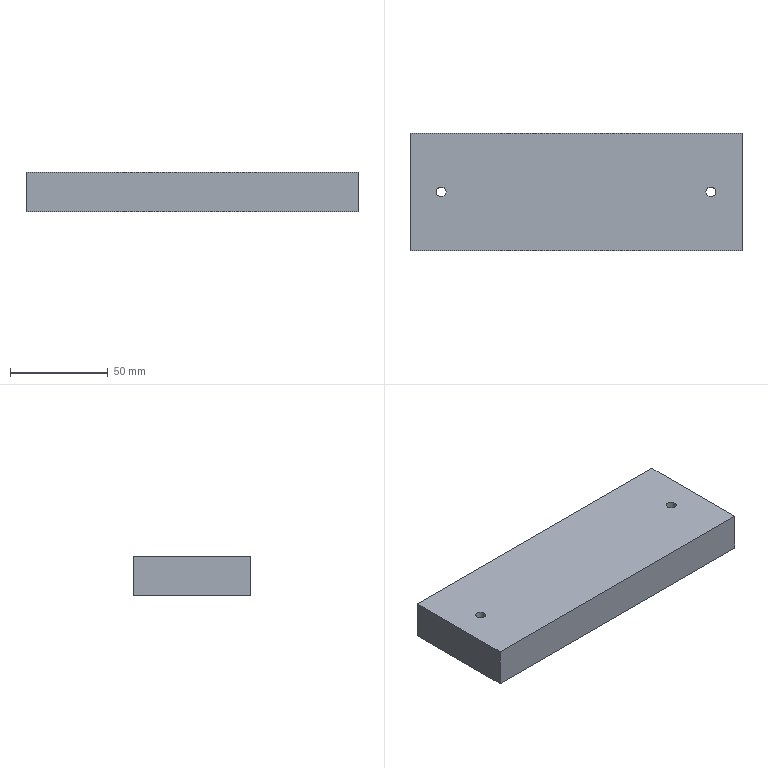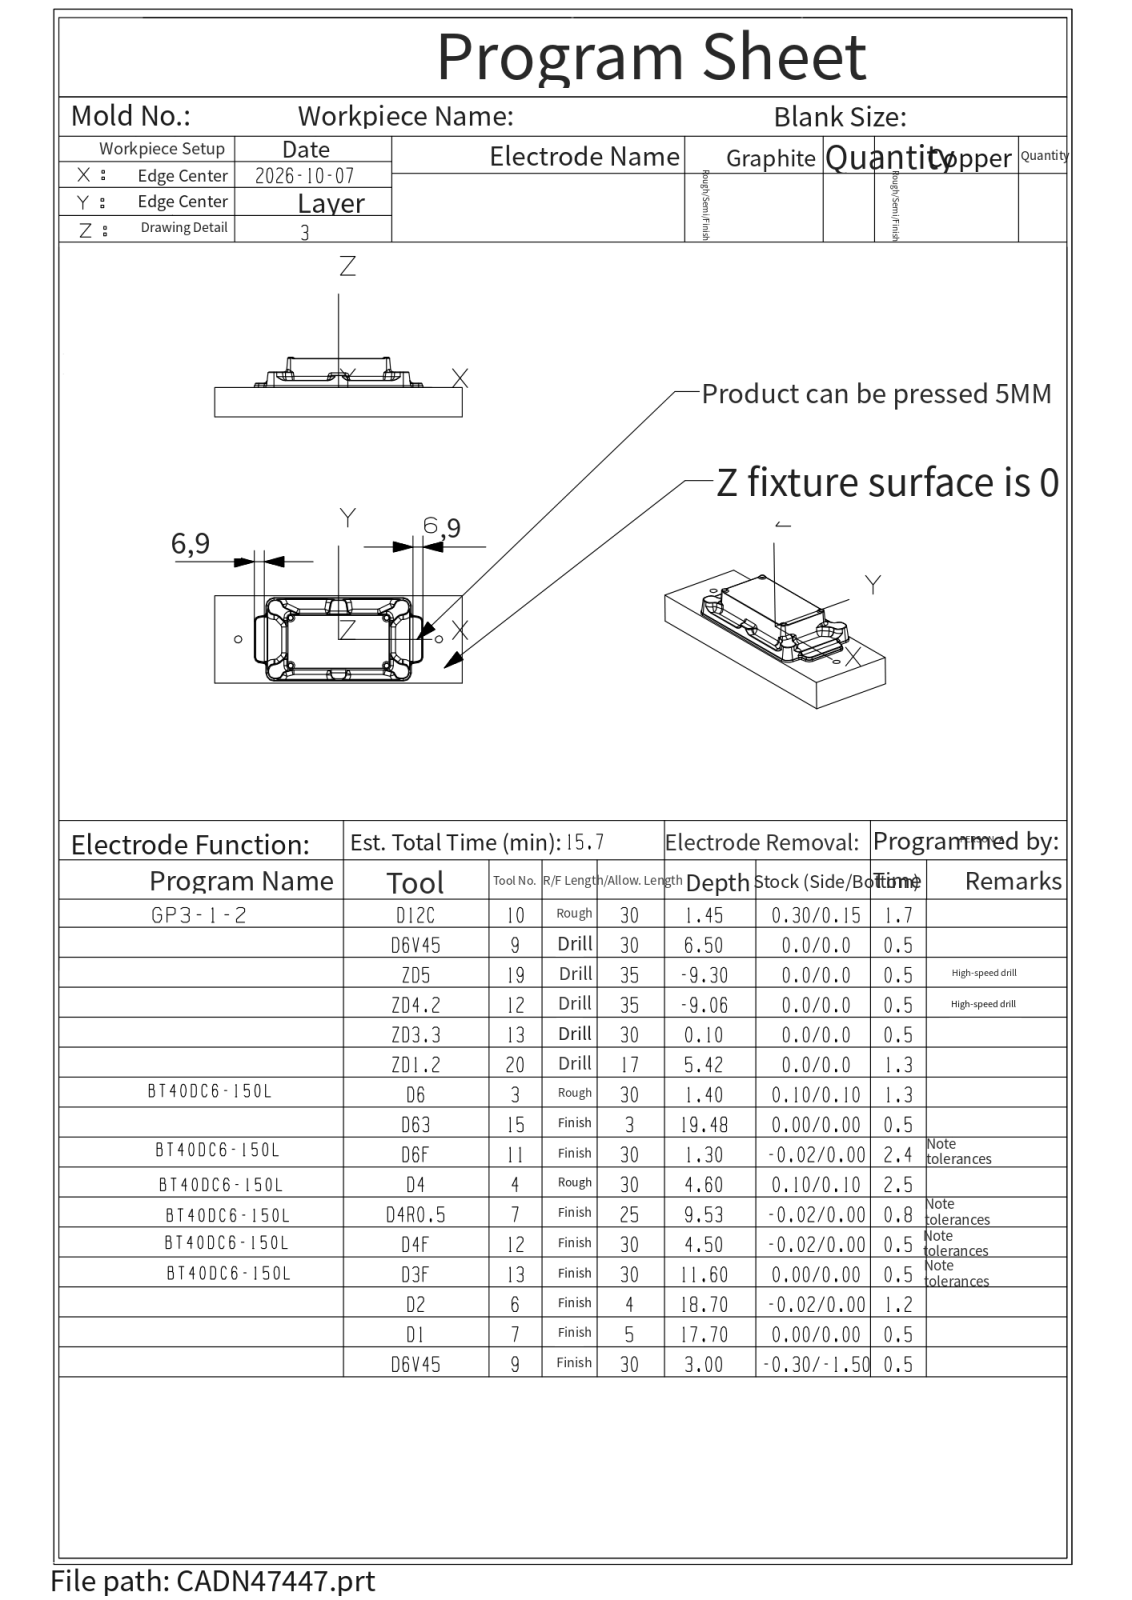NC program | NX | posted by the shop | part box 170 x 60 x 20 mm
Lines 1923 to 2905 of 17682:
T04 M06
T05
( name=D4    T=4 )
( XY = 0.10 )
( Z = 0.10 )
G00 G90 G54 X-4. Y-48. S10000 M03
G43 Z27.98 H04 M08
Z18.48
G03 X-3.5 I.25 J0.0 F4000.
G01 X-3.521 Y-47.848 Z18.47 F5000.
X-3.589 Y-47.71 Z18.46
X-3.696 Y-47.599 Z18.451
X-3.832 Y-47.526 Z18.441
X-3.984 Y-47.497 Z18.431
X-4.137 Y-47.516 Z18.421
X-4.277 Y-47.58 Z18.411
X-4.391 Y-47.684 Z18.402
X-4.469 Y-47.817 Z18.392
X-4.502 Y-47.967 Z18.382
X-4.488 Y-48.121 Z18.372
X-4.429 Y-48.263 Z18.362
X-4.329 Y-48.381 Z18.353
X-4.198 Y-48.462 Z18.343
X-4.049 Y-48.501 Z18.333
X-3.895 Y-48.492 Z18.323
X-3.751 Y-48.437 Z18.314
X-3.63 Y-48.341 Z18.304
X-3.544 Y-48.213 Z18.294
X-3.501 Y-48.065 Z18.284
X-3.505 Y-47.911 Z18.274
X-3.555 Y-47.765 Z18.265
X-3.647 Y-47.641 Z18.255
X-3.772 Y-47.551 Z18.245
X-3.919 Y-47.504 Z18.235
X-4.073 Y-47.502 Z18.225
X-4.22 Y-47.548 Z18.216
X-4.347 Y-47.636 Z18.206
X-4.441 Y-47.758 Z18.196
X-4.494 Y-47.903 Z18.186
X-4.5 Y-48.057 Z18.176
X-4.459 Y-48.206 Z18.167
X-4.375 Y-48.335 Z18.157
X-4.256 Y-48.433 Z18.147
X-4.113 Y-48.49 Z18.137
X-3.959 Y-48.501 Z18.127
X-3.809 Y-48.465 Z18.118
X-3.677 Y-48.386 Z18.108
X-3.576 Y-48.27 Z18.098
X-3.514 Y-48.129 Z18.088
X-3.498 Y-47.976 Z18.078
X-3.529 Y-47.825 Z18.069
X-3.604 Y-47.69 Z18.059
X-3.716 Y-47.585 Z18.049
X-3.855 Y-47.518 Z18.039
X-4.008 Y-47.497 Z18.029
X-4.16 Y-47.523 Z18.02
X-4.297 Y-47.594 Z18.01
X-4.406 Y-47.703 Z18.
X-4.477 Y-47.84 Z17.99
X-4.503 Y-47.992 Z17.981
X-4.482 Y-48.145 Z17.971
X-4.415 Y-48.284 Z17.961
X-4.31 Y-48.396 Z17.951
X-4.175 Y-48.471 Z17.941
X-4.024 Y-48.502 Z17.932
X-3.871 Y-48.486 Z17.922
X-3.73 Y-48.424 Z17.912
X-3.614 Y-48.323 Z17.902
X-3.535 Y-48.191 Z17.892
X-3.499 Y-48.041 Z17.883
X-3.51 Y-47.887 Z17.873
X-3.567 Y-47.744 Z17.863
X-3.665 Y-47.625 Z17.853
X-3.794 Y-47.541 Z17.843
X-3.943 Y-47.5 Z17.834
X-4.097 Y-47.506 Z17.824
X-4.242 Y-47.559 Z17.814
X-4.364 Y-47.653 Z17.804
X-4.452 Y-47.78 Z17.794
X-4.498 Y-47.927 Z17.785
X-4.496 Y-48.081 Z17.775
X-4.449 Y-48.228 Z17.765
X-4.359 Y-48.353 Z17.755
X-4.235 Y-48.445 Z17.745
X-4.089 Y-48.495 Z17.736
X-3.935 Y-48.499 Z17.726
X-3.787 Y-48.456 Z17.716
X-3.659 Y-48.37 Z17.706
X-3.563 Y-48.249 Z17.697
X-3.508 Y-48.105 Z17.687
X-3.499 Y-47.951 Z17.677
X-3.538 Y-47.802 Z17.667
X-3.619 Y-47.671 Z17.657
X-3.737 Y-47.571 Z17.648
X-3.879 Y-47.512 Z17.638
X-4.033 Y-47.498 Z17.628
X-4.183 Y-47.531 Z17.618
X-4.316 Y-47.609 Z17.608
X-4.42 Y-47.723 Z17.599
X-4.484 Y-47.863 Z17.589
X-4.503 Y-48.016 Z17.579
X-4.474 Y-48.168 Z17.569
X-4.401 Y-48.304 Z17.559
X-4.29 Y-48.411 Z17.55
X-4.152 Y-48.479 Z17.54
X-4. Y-48.503 Z17.53
X-3.848 Y-48.479 Z17.52
X-3.71 Y-48.411 Z17.51
X-3.599 Y-48.304 Z17.501
X-3.526 Y-48.168 Z17.491
X-3.497 Y-48.016 Z17.481
X-3.516 Y-47.863 Z17.471
X-3.58 Y-47.723 Z17.461
X-3.684 Y-47.609 Z17.452
X-3.817 Y-47.531 Z17.442
X-3.967 Y-47.498 Z17.432
X-4.121 Y-47.512 Z17.422
X-4.263 Y-47.571 Z17.412
X-4.381 Y-47.671 Z17.403
X-4.462 Y-47.802 Z17.393
X-4.501 Y-47.951 Z17.383
X-4.492 Y-48.105 Z17.373
X-4.437 Y-48.249 Z17.364
X-4.341 Y-48.37 Z17.354
X-4.213 Y-48.456 Z17.344
X-4.065 Y-48.499 Z17.334
X-3.911 Y-48.495 Z17.324
X-3.765 Y-48.445 Z17.315
X-3.641 Y-48.353 Z17.305
X-3.551 Y-48.228 Z17.295
X-3.504 Y-48.081 Z17.285
X-3.502 Y-47.927 Z17.275
X-3.548 Y-47.78 Z17.266
X-3.636 Y-47.653 Z17.256
X-3.758 Y-47.559 Z17.246
X-3.903 Y-47.506 Z17.236
X-4.057 Y-47.5 Z17.226
X-4.206 Y-47.541 Z17.217
X-4.335 Y-47.625 Z17.207
X-4.433 Y-47.744 Z17.197
X-4.49 Y-47.887 Z17.187
X-4.501 Y-48.041 Z17.177
X-4.465 Y-48.191 Z17.168
X-4.386 Y-48.323 Z17.158
X-4.27 Y-48.424 Z17.148
X-4.129 Y-48.486 Z17.138
X-3.976 Y-48.502 Z17.128
X-3.825 Y-48.471 Z17.119
X-3.69 Y-48.396 Z17.109
X-3.585 Y-48.284 Z17.099
X-3.518 Y-48.145 Z17.089
X-3.497 Y-47.992 Z17.079
X-3.523 Y-47.84 Z17.07
X-3.594 Y-47.703 Z17.06
X-3.703 Y-47.594 Z17.05
X-3.84 Y-47.523 Z17.04
X-3.992 Y-47.497 Z17.031
X-4.145 Y-47.518 Z17.021
X-4.284 Y-47.585 Z17.011
X-4.396 Y-47.69 Z17.001
X-4.471 Y-47.825 Z16.991
X-4.502 Y-47.976 Z16.982
X-4.486 Y-48.129 Z16.972
X-4.424 Y-48.27 Z16.962
X-4.323 Y-48.386 Z16.952
X-4.191 Y-48.465 Z16.942
X-4.041 Y-48.501 Z16.933
X-3.887 Y-48.49 Z16.923
X-3.744 Y-48.433 Z16.913
X-3.625 Y-48.335 Z16.903
X-3.541 Y-48.206 Z16.893
X-3.5 Y-48.057 Z16.884
X-3.506 Y-47.903 Z16.874
X-3.559 Y-47.758 Z16.864
X-3.653 Y-47.636 Z16.854
X-3.78 Y-47.548 Z16.844
X-3.927 Y-47.502 Z16.835
X-4.081 Y-47.504 Z16.825
X-4.228 Y-47.551 Z16.815
X-4.353 Y-47.641 Z16.805
X-4.445 Y-47.765 Z16.795
X-4.495 Y-47.911 Z16.786
X-4.499 Y-48.065 Z16.776
X-4.456 Y-48.213 Z16.766
X-4.37 Y-48.341 Z16.756
X-4.249 Y-48.437 Z16.747
X-4.105 Y-48.492 Z16.737
X-3.951 Y-48.501 Z16.727
X-3.802 Y-48.462 Z16.717
X-3.671 Y-48.381 Z16.707
X-3.571 Y-48.263 Z16.698
X-3.512 Y-48.121 Z16.688
X-3.498 Y-47.967 Z16.678
X-3.531 Y-47.817 Z16.668
X-3.609 Y-47.684 Z16.658
X-3.723 Y-47.58 Z16.649
X-3.863 Y-47.516 Z16.639
X-4.016 Y-47.497 Z16.629
X-4.168 Y-47.526 Z16.619
X-4.304 Y-47.599 Z16.609
X-4.411 Y-47.71 Z16.6
X-4.479 Y-47.848 Z16.59
X-4.5 Y-48. Z16.58
G03 I.5 J0.0
X-4. I.25 J0.0
G00 Z26.5
G01 Y-4. F6000.
G00 Z18.48
G03 X-3.5 I.25 J0.0 F4000.
G01 X-3.521 Y-3.848 Z18.47 F5000.
X-3.589 Y-3.71 Z18.46
X-3.696 Y-3.599 Z18.451
X-3.832 Y-3.526 Z18.441
X-3.984 Y-3.497 Z18.431
X-4.137 Y-3.516 Z18.421
X-4.277 Y-3.58 Z18.411
X-4.391 Y-3.684 Z18.402
X-4.469 Y-3.817 Z18.392
X-4.502 Y-3.967 Z18.382
X-4.488 Y-4.121 Z18.372
X-4.429 Y-4.263 Z18.362
X-4.329 Y-4.381 Z18.353
X-4.198 Y-4.462 Z18.343
X-4.049 Y-4.501 Z18.333
X-3.895 Y-4.492 Z18.323
X-3.751 Y-4.437 Z18.314
X-3.63 Y-4.341 Z18.304
X-3.544 Y-4.213 Z18.294
X-3.501 Y-4.065 Z18.284
X-3.505 Y-3.911 Z18.274
X-3.555 Y-3.765 Z18.265
X-3.647 Y-3.641 Z18.255
X-3.772 Y-3.551 Z18.245
X-3.919 Y-3.504 Z18.235
X-4.073 Y-3.502 Z18.225
X-4.22 Y-3.548 Z18.216
X-4.347 Y-3.636 Z18.206
X-4.441 Y-3.758 Z18.196
X-4.494 Y-3.903 Z18.186
X-4.5 Y-4.057 Z18.176
X-4.459 Y-4.206 Z18.167
X-4.375 Y-4.335 Z18.157
X-4.256 Y-4.433 Z18.147
X-4.113 Y-4.49 Z18.137
X-3.959 Y-4.501 Z18.127
X-3.809 Y-4.465 Z18.118
X-3.677 Y-4.386 Z18.108
X-3.576 Y-4.27 Z18.098
X-3.514 Y-4.129 Z18.088
X-3.498 Y-3.976 Z18.078
X-3.529 Y-3.825 Z18.069
X-3.604 Y-3.69 Z18.059
X-3.716 Y-3.585 Z18.049
X-3.855 Y-3.518 Z18.039
X-4.008 Y-3.497 Z18.029
X-4.16 Y-3.523 Z18.02
X-4.297 Y-3.594 Z18.01
X-4.406 Y-3.703 Z18.
X-4.477 Y-3.84 Z17.99
X-4.503 Y-3.992 Z17.981
X-4.482 Y-4.145 Z17.971
X-4.415 Y-4.284 Z17.961
X-4.31 Y-4.396 Z17.951
X-4.175 Y-4.471 Z17.941
X-4.024 Y-4.502 Z17.932
X-3.871 Y-4.486 Z17.922
X-3.73 Y-4.424 Z17.912
X-3.614 Y-4.323 Z17.902
X-3.535 Y-4.191 Z17.892
X-3.499 Y-4.041 Z17.883
X-3.51 Y-3.887 Z17.873
X-3.567 Y-3.744 Z17.863
X-3.665 Y-3.625 Z17.853
X-3.794 Y-3.541 Z17.843
X-3.943 Y-3.5 Z17.834
X-4.097 Y-3.506 Z17.824
X-4.242 Y-3.559 Z17.814
X-4.364 Y-3.653 Z17.804
X-4.452 Y-3.78 Z17.794
X-4.498 Y-3.927 Z17.785
X-4.496 Y-4.081 Z17.775
X-4.449 Y-4.228 Z17.765
X-4.359 Y-4.353 Z17.755
X-4.235 Y-4.445 Z17.745
X-4.089 Y-4.495 Z17.736
X-3.935 Y-4.499 Z17.726
X-3.787 Y-4.456 Z17.716
X-3.659 Y-4.37 Z17.706
X-3.563 Y-4.249 Z17.697
X-3.508 Y-4.105 Z17.687
X-3.499 Y-3.951 Z17.677
X-3.538 Y-3.802 Z17.667
X-3.619 Y-3.671 Z17.657
X-3.737 Y-3.571 Z17.648
X-3.879 Y-3.512 Z17.638
X-4.033 Y-3.498 Z17.628
X-4.183 Y-3.531 Z17.618
X-4.316 Y-3.609 Z17.608
X-4.42 Y-3.723 Z17.599
X-4.484 Y-3.863 Z17.589
X-4.503 Y-4.016 Z17.579
X-4.474 Y-4.168 Z17.569
X-4.401 Y-4.304 Z17.559
X-4.29 Y-4.411 Z17.55
X-4.152 Y-4.479 Z17.54
X-4. Y-4.503 Z17.53
X-3.848 Y-4.479 Z17.52
X-3.71 Y-4.411 Z17.51
X-3.599 Y-4.304 Z17.501
X-3.526 Y-4.168 Z17.491
X-3.497 Y-4.016 Z17.481
X-3.516 Y-3.863 Z17.471
X-3.58 Y-3.723 Z17.461
X-3.684 Y-3.609 Z17.452
X-3.817 Y-3.531 Z17.442
X-3.967 Y-3.498 Z17.432
X-4.121 Y-3.512 Z17.422
X-4.263 Y-3.571 Z17.412
X-4.381 Y-3.671 Z17.403
X-4.462 Y-3.802 Z17.393
X-4.501 Y-3.951 Z17.383
X-4.492 Y-4.105 Z17.373
X-4.437 Y-4.249 Z17.364
X-4.341 Y-4.37 Z17.354
X-4.213 Y-4.456 Z17.344
X-4.065 Y-4.499 Z17.334
X-3.911 Y-4.495 Z17.324
X-3.765 Y-4.445 Z17.315
X-3.641 Y-4.353 Z17.305
X-3.551 Y-4.228 Z17.295
X-3.504 Y-4.081 Z17.285
X-3.502 Y-3.927 Z17.275
X-3.548 Y-3.78 Z17.266
X-3.636 Y-3.653 Z17.256
X-3.758 Y-3.559 Z17.246
X-3.903 Y-3.506 Z17.236
X-4.057 Y-3.5 Z17.226
X-4.206 Y-3.541 Z17.217
X-4.335 Y-3.625 Z17.207
X-4.433 Y-3.744 Z17.197
X-4.49 Y-3.887 Z17.187
X-4.501 Y-4.041 Z17.177
X-4.465 Y-4.191 Z17.168
X-4.386 Y-4.323 Z17.158
X-4.27 Y-4.424 Z17.148
X-4.129 Y-4.486 Z17.138
X-3.976 Y-4.502 Z17.128
X-3.825 Y-4.471 Z17.119
X-3.69 Y-4.396 Z17.109
X-3.585 Y-4.284 Z17.099
X-3.518 Y-4.145 Z17.089
X-3.497 Y-3.992 Z17.079
X-3.523 Y-3.84 Z17.07
X-3.594 Y-3.703 Z17.06
X-3.703 Y-3.594 Z17.05
X-3.84 Y-3.523 Z17.04
X-3.992 Y-3.497 Z17.031
X-4.145 Y-3.518 Z17.021
X-4.284 Y-3.585 Z17.011
X-4.396 Y-3.69 Z17.001
X-4.471 Y-3.825 Z16.991
X-4.502 Y-3.976 Z16.982
X-4.486 Y-4.129 Z16.972
X-4.424 Y-4.27 Z16.962
X-4.323 Y-4.386 Z16.952
X-4.191 Y-4.465 Z16.942
X-4.041 Y-4.501 Z16.933
X-3.887 Y-4.49 Z16.923
X-3.744 Y-4.433 Z16.913
X-3.625 Y-4.335 Z16.903
X-3.541 Y-4.206 Z16.893
X-3.5 Y-4.057 Z16.884
X-3.506 Y-3.903 Z16.874
X-3.559 Y-3.758 Z16.864
X-3.653 Y-3.636 Z16.854
X-3.78 Y-3.548 Z16.844
X-3.927 Y-3.502 Z16.835
X-4.081 Y-3.504 Z16.825
X-4.228 Y-3.551 Z16.815
X-4.353 Y-3.641 Z16.805
X-4.445 Y-3.765 Z16.795
X-4.495 Y-3.911 Z16.786
X-4.499 Y-4.065 Z16.776
X-4.456 Y-4.213 Z16.766
X-4.37 Y-4.341 Z16.756
X-4.249 Y-4.437 Z16.747
X-4.105 Y-4.492 Z16.737
X-3.951 Y-4.501 Z16.727
X-3.802 Y-4.462 Z16.717
X-3.671 Y-4.381 Z16.707
X-3.571 Y-4.263 Z16.698
X-3.512 Y-4.121 Z16.688
X-3.498 Y-3.967 Z16.678
X-3.531 Y-3.817 Z16.668
X-3.609 Y-3.684 Z16.658
X-3.723 Y-3.58 Z16.649
X-3.863 Y-3.516 Z16.639
X-4.016 Y-3.497 Z16.629
X-4.168 Y-3.526 Z16.619
X-4.304 Y-3.599 Z16.609
X-4.411 Y-3.71 Z16.6
X-4.479 Y-3.848 Z16.59
X-4.5 Y-4. Z16.58
G03 I.5 J0.0
X-4. I.25 J0.0
G00 Z26.5
G01 X-47.4 F6000.
G00 Z18.48
G03 X-46.9 I.25 J0.0 F4000.
G01 X-46.921 Y-3.848 Z18.47 F5000.
X-46.989 Y-3.71 Z18.46
X-47.096 Y-3.599 Z18.451
X-47.232 Y-3.526 Z18.441
X-47.384 Y-3.497 Z18.431
X-47.537 Y-3.516 Z18.421
X-47.677 Y-3.58 Z18.411
X-47.791 Y-3.684 Z18.402
X-47.869 Y-3.817 Z18.392
X-47.902 Y-3.967 Z18.382
X-47.888 Y-4.121 Z18.372
X-47.829 Y-4.263 Z18.362
X-47.729 Y-4.381 Z18.353
X-47.598 Y-4.462 Z18.343
X-47.449 Y-4.501 Z18.333
X-47.295 Y-4.492 Z18.323
X-47.151 Y-4.437 Z18.314
X-47.03 Y-4.341 Z18.304
X-46.944 Y-4.213 Z18.294
X-46.901 Y-4.065 Z18.284
X-46.905 Y-3.911 Z18.274
X-46.955 Y-3.765 Z18.265
X-47.047 Y-3.641 Z18.255
X-47.172 Y-3.551 Z18.245
X-47.319 Y-3.504 Z18.235
X-47.473 Y-3.502 Z18.225
X-47.62 Y-3.548 Z18.216
X-47.747 Y-3.636 Z18.206
X-47.841 Y-3.758 Z18.196
X-47.894 Y-3.903 Z18.186
X-47.9 Y-4.057 Z18.176
X-47.859 Y-4.206 Z18.167
X-47.775 Y-4.335 Z18.157
X-47.656 Y-4.433 Z18.147
X-47.513 Y-4.49 Z18.137
X-47.359 Y-4.501 Z18.127
X-47.209 Y-4.465 Z18.118
X-47.077 Y-4.386 Z18.108
X-46.976 Y-4.27 Z18.098
X-46.914 Y-4.129 Z18.088
X-46.898 Y-3.976 Z18.078
X-46.929 Y-3.825 Z18.069
X-47.004 Y-3.69 Z18.059
X-47.116 Y-3.585 Z18.049
X-47.255 Y-3.518 Z18.039
X-47.408 Y-3.497 Z18.029
X-47.56 Y-3.523 Z18.02
X-47.697 Y-3.594 Z18.01
X-47.806 Y-3.703 Z18.
X-47.877 Y-3.84 Z17.99
X-47.903 Y-3.992 Z17.981
X-47.882 Y-4.145 Z17.971
X-47.815 Y-4.284 Z17.961
X-47.71 Y-4.396 Z17.951
X-47.575 Y-4.471 Z17.941
X-47.424 Y-4.502 Z17.932
X-47.271 Y-4.486 Z17.922
X-47.13 Y-4.424 Z17.912
X-47.014 Y-4.323 Z17.902
X-46.935 Y-4.191 Z17.892
X-46.899 Y-4.041 Z17.883
X-46.91 Y-3.887 Z17.873
X-46.967 Y-3.744 Z17.863
X-47.065 Y-3.625 Z17.853
X-47.194 Y-3.541 Z17.843
X-47.343 Y-3.5 Z17.834
X-47.497 Y-3.506 Z17.824
X-47.642 Y-3.559 Z17.814
X-47.764 Y-3.653 Z17.804
X-47.852 Y-3.78 Z17.794
X-47.898 Y-3.927 Z17.785
X-47.896 Y-4.081 Z17.775
X-47.849 Y-4.228 Z17.765
X-47.759 Y-4.353 Z17.755
X-47.635 Y-4.445 Z17.745
X-47.489 Y-4.495 Z17.736
X-47.335 Y-4.499 Z17.726
X-47.187 Y-4.456 Z17.716
X-47.059 Y-4.37 Z17.706
X-46.963 Y-4.249 Z17.697
X-46.908 Y-4.105 Z17.687
X-46.899 Y-3.951 Z17.677
X-46.938 Y-3.802 Z17.667
X-47.019 Y-3.671 Z17.657
X-47.137 Y-3.571 Z17.648
X-47.279 Y-3.512 Z17.638
X-47.433 Y-3.498 Z17.628
X-47.583 Y-3.531 Z17.618
X-47.716 Y-3.609 Z17.608
X-47.82 Y-3.723 Z17.599
X-47.884 Y-3.863 Z17.589
X-47.903 Y-4.016 Z17.579
X-47.874 Y-4.168 Z17.569
X-47.801 Y-4.304 Z17.559
X-47.69 Y-4.411 Z17.55
X-47.552 Y-4.479 Z17.54
X-47.4 Y-4.503 Z17.53
X-47.248 Y-4.479 Z17.52
X-47.11 Y-4.411 Z17.51
X-46.999 Y-4.304 Z17.501
X-46.926 Y-4.168 Z17.491
X-46.897 Y-4.016 Z17.481
X-46.916 Y-3.863 Z17.471
X-46.98 Y-3.723 Z17.461
X-47.084 Y-3.609 Z17.452
X-47.217 Y-3.531 Z17.442
X-47.367 Y-3.498 Z17.432
X-47.521 Y-3.512 Z17.422
X-47.663 Y-3.571 Z17.412
X-47.781 Y-3.671 Z17.403
X-47.862 Y-3.802 Z17.393
X-47.901 Y-3.951 Z17.383
X-47.892 Y-4.105 Z17.373
X-47.837 Y-4.249 Z17.364
X-47.741 Y-4.37 Z17.354
X-47.613 Y-4.456 Z17.344
X-47.465 Y-4.499 Z17.334
X-47.311 Y-4.495 Z17.324
X-47.165 Y-4.445 Z17.315
X-47.041 Y-4.353 Z17.305
X-46.951 Y-4.228 Z17.295
X-46.904 Y-4.081 Z17.285
X-46.902 Y-3.927 Z17.275
X-46.948 Y-3.78 Z17.266
X-47.036 Y-3.653 Z17.256
X-47.158 Y-3.559 Z17.246
X-47.303 Y-3.506 Z17.236
X-47.457 Y-3.5 Z17.226
X-47.606 Y-3.541 Z17.217
X-47.735 Y-3.625 Z17.207
X-47.833 Y-3.744 Z17.197
X-47.89 Y-3.887 Z17.187
X-47.901 Y-4.041 Z17.177
X-47.865 Y-4.191 Z17.168
X-47.786 Y-4.323 Z17.158
X-47.67 Y-4.424 Z17.148
X-47.529 Y-4.486 Z17.138
X-47.376 Y-4.502 Z17.128
X-47.225 Y-4.471 Z17.119
X-47.09 Y-4.396 Z17.109
X-46.985 Y-4.284 Z17.099
X-46.918 Y-4.145 Z17.089
X-46.897 Y-3.992 Z17.079
X-46.923 Y-3.84 Z17.07
X-46.994 Y-3.703 Z17.06
X-47.103 Y-3.594 Z17.05
X-47.24 Y-3.523 Z17.04
X-47.392 Y-3.497 Z17.031
X-47.545 Y-3.518 Z17.021
X-47.684 Y-3.585 Z17.011
X-47.796 Y-3.69 Z17.001
X-47.871 Y-3.825 Z16.991
X-47.902 Y-3.976 Z16.982
X-47.886 Y-4.129 Z16.972
X-47.824 Y-4.27 Z16.962
X-47.723 Y-4.386 Z16.952
X-47.591 Y-4.465 Z16.942
X-47.441 Y-4.501 Z16.933
X-47.287 Y-4.49 Z16.923
X-47.144 Y-4.433 Z16.913
X-47.025 Y-4.335 Z16.903
X-46.941 Y-4.206 Z16.893
X-46.9 Y-4.057 Z16.884
X-46.906 Y-3.903 Z16.874
X-46.959 Y-3.758 Z16.864
X-47.053 Y-3.636 Z16.854
X-47.18 Y-3.548 Z16.844
X-47.327 Y-3.502 Z16.835
X-47.481 Y-3.504 Z16.825
X-47.628 Y-3.551 Z16.815
X-47.753 Y-3.641 Z16.805
X-47.845 Y-3.765 Z16.795
X-47.895 Y-3.911 Z16.786
X-47.899 Y-4.065 Z16.776
X-47.856 Y-4.213 Z16.766
X-47.77 Y-4.341 Z16.756
X-47.649 Y-4.437 Z16.747
X-47.505 Y-4.492 Z16.737
X-47.351 Y-4.501 Z16.727
X-47.202 Y-4.462 Z16.717
X-47.071 Y-4.381 Z16.707
X-46.971 Y-4.263 Z16.698
X-46.912 Y-4.121 Z16.688
X-46.898 Y-3.967 Z16.678
X-46.931 Y-3.817 Z16.668
X-47.009 Y-3.684 Z16.658
X-47.123 Y-3.58 Z16.649
X-47.263 Y-3.516 Z16.639
X-47.416 Y-3.497 Z16.629
X-47.568 Y-3.526 Z16.619
X-47.704 Y-3.599 Z16.609
X-47.811 Y-3.71 Z16.6
X-47.879 Y-3.848 Z16.59
X-47.9 Y-4. Z16.58
G03 I.5 J0.0
X-47.4 I.25 J0.0
G00 Z26.5
G01 X-90.8 F6000.
G00 Z18.48
G03 X-90.3 I.25 J0.0 F4000.
G01 X-90.321 Y-3.848 Z18.47 F5000.
X-90.389 Y-3.71 Z18.46
X-90.496 Y-3.599 Z18.451
X-90.632 Y-3.526 Z18.441
X-90.784 Y-3.497 Z18.431
X-90.937 Y-3.516 Z18.421
X-91.077 Y-3.58 Z18.411
X-91.191 Y-3.684 Z18.402
X-91.269 Y-3.817 Z18.392
X-91.302 Y-3.967 Z18.382
X-91.288 Y-4.121 Z18.372
X-91.229 Y-4.263 Z18.362
X-91.129 Y-4.381 Z18.353
X-90.998 Y-4.462 Z18.343
X-90.849 Y-4.501 Z18.333
X-90.695 Y-4.492 Z18.323
X-90.551 Y-4.437 Z18.314
X-90.43 Y-4.341 Z18.304
X-90.344 Y-4.213 Z18.294
X-90.301 Y-4.065 Z18.284
X-90.305 Y-3.911 Z18.274
X-90.355 Y-3.765 Z18.265
X-90.447 Y-3.641 Z18.255
X-90.572 Y-3.551 Z18.245
X-90.719 Y-3.504 Z18.235
X-90.873 Y-3.502 Z18.225
X-91.02 Y-3.548 Z18.216
X-91.147 Y-3.636 Z18.206
X-91.241 Y-3.758 Z18.196
X-91.294 Y-3.903 Z18.186
X-91.3 Y-4.057 Z18.176
X-91.259 Y-4.206 Z18.167
X-91.175 Y-4.335 Z18.157
X-91.056 Y-4.433 Z18.147
X-90.913 Y-4.49 Z18.137
X-90.759 Y-4.501 Z18.127
X-90.609 Y-4.465 Z18.118
X-90.477 Y-4.386 Z18.108
X-90.376 Y-4.27 Z18.098
X-90.314 Y-4.129 Z18.088
X-90.298 Y-3.976 Z18.078
X-90.329 Y-3.825 Z18.069
X-90.404 Y-3.69 Z18.059
X-90.516 Y-3.585 Z18.049
X-90.655 Y-3.518 Z18.039
X-90.808 Y-3.497 Z18.029
X-90.96 Y-3.523 Z18.02
X-91.097 Y-3.594 Z18.01
X-91.206 Y-3.703 Z18.
X-91.277 Y-3.84 Z17.99
X-91.303 Y-3.992 Z17.981
X-91.282 Y-4.145 Z17.971
X-91.215 Y-4.284 Z17.961
X-91.11 Y-4.396 Z17.951
X-90.975 Y-4.471 Z17.941
X-90.824 Y-4.502 Z17.932
X-90.671 Y-4.486 Z17.922
X-90.53 Y-4.424 Z17.912
X-90.414 Y-4.323 Z17.902
X-90.335 Y-4.191 Z17.892
X-90.299 Y-4.041 Z17.883
X-90.31 Y-3.887 Z17.873
X-90.367 Y-3.744 Z17.863
X-90.465 Y-3.625 Z17.853
X-90.594 Y-3.541 Z17.843
X-90.743 Y-3.5 Z17.834
X-90.897 Y-3.506 Z17.824
X-91.042 Y-3.559 Z17.814
X-91.164 Y-3.653 Z17.804
X-91.252 Y-3.78 Z17.794
X-91.298 Y-3.927 Z17.785
X-91.296 Y-4.081 Z17.775
X-91.249 Y-4.228 Z17.765
X-91.159 Y-4.353 Z17.755
X-91.035 Y-4.445 Z17.745
X-90.889 Y-4.495 Z17.736
X-90.735 Y-4.499 Z17.726
X-90.587 Y-4.456 Z17.716
X-90.459 Y-4.37 Z17.706
X-90.363 Y-4.249 Z17.697
X-90.308 Y-4.105 Z17.687
X-90.299 Y-3.951 Z17.677
X-90.338 Y-3.802 Z17.667
X-90.419 Y-3.671 Z17.657
X-90.537 Y-3.571 Z17.648
X-90.679 Y-3.512 Z17.638
X-90.833 Y-3.498 Z17.628
X-90.983 Y-3.531 Z17.618
X-91.116 Y-3.609 Z17.608
X-91.22 Y-3.723 Z17.599
X-91.284 Y-3.863 Z17.589
X-91.303 Y-4.016 Z17.579
X-91.274 Y-4.168 Z17.569
X-91.201 Y-4.304 Z17.559
X-91.09 Y-4.411 Z17.55
X-90.952 Y-4.479 Z17.54
X-90.8 Y-4.503 Z17.53
X-90.648 Y-4.479 Z17.52
X-90.51 Y-4.411 Z17.51
X-90.399 Y-4.304 Z17.501
X-90.326 Y-4.168 Z17.491
X-90.297 Y-4.016 Z17.481
X-90.316 Y-3.863 Z17.471
X-90.38 Y-3.723 Z17.461
X-90.484 Y-3.609 Z17.452
X-90.617 Y-3.531 Z17.442
X-90.767 Y-3.498 Z17.432
X-90.921 Y-3.512 Z17.422
X-91.063 Y-3.571 Z17.412
X-91.181 Y-3.671 Z17.403
X-91.262 Y-3.802 Z17.393
X-91.301 Y-3.951 Z17.383
X-91.292 Y-4.105 Z17.373
X-91.237 Y-4.249 Z17.364
X-91.141 Y-4.37 Z17.354
X-91.013 Y-4.456 Z17.344
X-90.865 Y-4.499 Z17.334
X-90.711 Y-4.495 Z17.324
X-90.565 Y-4.445 Z17.315
X-90.441 Y-4.353 Z17.305
X-90.351 Y-4.228 Z17.295
X-90.304 Y-4.081 Z17.285
X-90.302 Y-3.927 Z17.275
X-90.348 Y-3.78 Z17.266
X-90.436 Y-3.653 Z17.256
X-90.558 Y-3.559 Z17.246
X-90.703 Y-3.506 Z17.236
X-90.857 Y-3.5 Z17.226
X-91.006 Y-3.541 Z17.217
X-91.135 Y-3.625 Z17.207
X-91.233 Y-3.744 Z17.197
X-91.29 Y-3.887 Z17.187
X-91.301 Y-4.041 Z17.177
X-91.265 Y-4.191 Z17.168
X-91.186 Y-4.323 Z17.158
X-91.07 Y-4.424 Z17.148
X-90.929 Y-4.486 Z17.138
X-90.776 Y-4.502 Z17.128
X-90.625 Y-4.471 Z17.119
X-90.49 Y-4.396 Z17.109
X-90.385 Y-4.284 Z17.099
X-90.318 Y-4.145 Z17.089
X-90.297 Y-3.992 Z17.079
X-90.323 Y-3.84 Z17.07
X-90.394 Y-3.703 Z17.06
X-90.503 Y-3.594 Z17.05
X-90.64 Y-3.523 Z17.04
X-90.792 Y-3.497 Z17.031
X-90.945 Y-3.518 Z17.021
X-91.084 Y-3.585 Z17.011
X-91.196 Y-3.69 Z17.001
X-91.271 Y-3.825 Z16.991
X-91.302 Y-3.976 Z16.982
X-91.286 Y-4.129 Z16.972
X-91.224 Y-4.27 Z16.962
X-91.123 Y-4.386 Z16.952
X-90.991 Y-4.465 Z16.942
X-90.841 Y-4.501 Z16.933
X-90.687 Y-4.49 Z16.923
X-90.544 Y-4.433 Z16.913
X-90.425 Y-4.335 Z16.903
X-90.341 Y-4.206 Z16.893
X-90.3 Y-4.057 Z16.884
X-90.306 Y-3.903 Z16.874
X-90.359 Y-3.758 Z16.864
X-90.453 Y-3.636 Z16.854
X-90.58 Y-3.548 Z16.844
X-90.727 Y-3.502 Z16.835
X-90.881 Y-3.504 Z16.825
X-91.028 Y-3.551 Z16.815
X-91.153 Y-3.641 Z16.805
X-91.245 Y-3.765 Z16.795
X-91.295 Y-3.911 Z16.786
X-91.299 Y-4.065 Z16.776
X-91.256 Y-4.213 Z16.766
X-91.17 Y-4.341 Z16.756
X-91.049 Y-4.437 Z16.747
X-90.905 Y-4.492 Z16.737
X-90.751 Y-4.501 Z16.727
X-90.602 Y-4.462 Z16.717
X-90.471 Y-4.381 Z16.707
X-90.371 Y-4.263 Z16.698
X-90.312 Y-4.121 Z16.688
X-90.298 Y-3.967 Z16.678
X-90.331 Y-3.817 Z16.668
X-90.409 Y-3.684 Z16.658
X-90.523 Y-3.58 Z16.649
X-90.663 Y-3.516 Z16.639
X-90.816 Y-3.497 Z16.629
X-90.968 Y-3.526 Z16.619
X-91.104 Y-3.599 Z16.609
X-91.211 Y-3.71 Z16.6
X-91.279 Y-3.848 Z16.59
X-91.3 Y-4. Z16.58
G03 I.5 J0.0
X-90.8 I.25 J0.0
G00 Z26.5
G01 Y-48. F6000.
G00 Z18.48
G03 X-90.3 I.25 J0.0 F4000.
G01 X-90.321 Y-47.848 Z18.47 F5000.
X-90.389 Y-47.71 Z18.46
X-90.496 Y-47.599 Z18.451
X-90.632 Y-47.526 Z18.441
X-90.784 Y-47.497 Z18.431
X-90.937 Y-47.516 Z18.421
X-91.077 Y-47.58 Z18.411
X-91.191 Y-47.684 Z18.402
X-91.269 Y-47.817 Z18.392
X-91.302 Y-47.967 Z18.382
X-91.288 Y-48.121 Z18.372
X-91.229 Y-48.263 Z18.362
X-91.129 Y-48.381 Z18.353
X-90.998 Y-48.462 Z18.343
X-90.849 Y-48.501 Z18.333
X-90.695 Y-48.492 Z18.323
X-90.551 Y-48.437 Z18.314
X-90.43 Y-48.341 Z18.304
X-90.344 Y-48.213 Z18.294
X-90.301 Y-48.065 Z18.284
X-90.305 Y-47.911 Z18.274
X-90.355 Y-47.765 Z18.265
X-90.447 Y-47.641 Z18.255
X-90.572 Y-47.551 Z18.245
X-90.719 Y-47.504 Z18.235
X-90.873 Y-47.502 Z18.225
X-91.02 Y-47.548 Z18.216
X-91.147 Y-47.636 Z18.206
X-91.241 Y-47.758 Z18.196
X-91.294 Y-47.903 Z18.186
X-91.3 Y-48.057 Z18.176
X-91.259 Y-48.206 Z18.167
X-91.175 Y-48.335 Z18.157
X-91.056 Y-48.433 Z18.147
X-90.913 Y-48.49 Z18.137
X-90.759 Y-48.501 Z18.127
X-90.609 Y-48.465 Z18.118
X-90.477 Y-48.386 Z18.108
X-90.376 Y-48.27 Z18.098
X-90.314 Y-48.129 Z18.088
X-90.298 Y-47.976 Z18.078
X-90.329 Y-47.825 Z18.069
X-90.404 Y-47.69 Z18.059
X-90.516 Y-47.585 Z18.049
X-90.655 Y-47.518 Z18.039
X-90.808 Y-47.497 Z18.029
X-90.96 Y-47.523 Z18.02
X-91.097 Y-47.594 Z18.01
X-91.206 Y-47.703 Z18.
X-91.277 Y-47.84 Z17.99
X-91.303 Y-47.992 Z17.981
X-91.282 Y-48.145 Z17.971
X-91.215 Y-48.284 Z17.961
X-91.11 Y-48.396 Z17.951
X-90.975 Y-48.471 Z17.941
X-90.824 Y-48.502 Z17.932
X-90.671 Y-48.486 Z17.922
X-90.53 Y-48.424 Z17.912
X-90.414 Y-48.323 Z17.902
X-90.335 Y-48.191 Z17.892
X-90.299 Y-48.041 Z17.883
X-90.31 Y-47.887 Z17.873
X-90.367 Y-47.744 Z17.863
X-90.465 Y-47.625 Z17.853
X-90.594 Y-47.541 Z17.843
X-90.743 Y-47.5 Z17.834
X-90.897 Y-47.506 Z17.824
X-91.042 Y-47.559 Z17.814
X-91.164 Y-47.653 Z17.804
X-91.252 Y-47.78 Z17.794
X-91.298 Y-47.927 Z17.785
X-91.296 Y-48.081 Z17.775
X-91.249 Y-48.228 Z17.765
X-91.159 Y-48.353 Z17.755
X-91.035 Y-48.445 Z17.745
X-90.889 Y-48.495 Z17.736
X-90.735 Y-48.499 Z17.726
X-90.587 Y-48.456 Z17.716
X-90.459 Y-48.37 Z17.706
X-90.363 Y-48.249 Z17.697
X-90.308 Y-48.105 Z17.687
X-90.299 Y-47.951 Z17.677
X-90.338 Y-47.802 Z17.667
X-90.419 Y-47.671 Z17.657
X-90.537 Y-47.571 Z17.648
X-90.679 Y-47.512 Z17.638
X-90.833 Y-47.498 Z17.628
X-90.983 Y-47.531 Z17.618
X-91.116 Y-47.609 Z17.608
X-91.22 Y-47.723 Z17.599
X-91.284 Y-47.863 Z17.589
X-91.303 Y-48.016 Z17.579
X-91.274 Y-48.168 Z17.569
X-91.201 Y-48.304 Z17.559
X-91.09 Y-48.411 Z17.55
X-90.952 Y-48.479 Z17.54
X-90.8 Y-48.503 Z17.53
X-90.648 Y-48.479 Z17.52
X-90.51 Y-48.411 Z17.51
X-90.399 Y-48.304 Z17.501
X-90.326 Y-48.168 Z17.491
X-90.297 Y-48.016 Z17.481
X-90.316 Y-47.863 Z17.471
X-90.38 Y-47.723 Z17.461
X-90.484 Y-47.609 Z17.452
X-90.617 Y-47.531 Z17.442
X-90.767 Y-47.498 Z17.432
X-90.921 Y-47.512 Z17.422
X-91.063 Y-47.571 Z17.412
X-91.181 Y-47.671 Z17.403
X-91.262 Y-47.802 Z17.393
X-91.301 Y-47.951 Z17.383
X-91.292 Y-48.105 Z17.373
X-91.237 Y-48.249 Z17.364
X-91.141 Y-48.37 Z17.354
X-91.013 Y-48.456 Z17.344
X-90.865 Y-48.499 Z17.334
X-90.711 Y-48.495 Z17.324
X-90.565 Y-48.445 Z17.315
X-90.441 Y-48.353 Z17.305
X-90.351 Y-48.228 Z17.295
X-90.304 Y-48.081 Z17.285
X-90.302 Y-47.927 Z17.275
X-90.348 Y-47.78 Z17.266
X-90.436 Y-47.653 Z17.256
X-90.558 Y-47.559 Z17.246
X-90.703 Y-47.506 Z17.236
X-90.857 Y-47.5 Z17.226
X-91.006 Y-47.541 Z17.217
X-91.135 Y-47.625 Z17.207
X-91.233 Y-47.744 Z17.197
X-91.29 Y-47.887 Z17.187
X-91.301 Y-48.041 Z17.177
X-91.265 Y-48.191 Z17.168
X-91.186 Y-48.323 Z17.158
X-91.07 Y-48.424 Z17.148
X-90.929 Y-48.486 Z17.138
X-90.776 Y-48.502 Z17.128
X-90.625 Y-48.471 Z17.119
X-90.49 Y-48.396 Z17.109
X-90.385 Y-48.284 Z17.099
X-90.318 Y-48.145 Z17.089
X-90.297 Y-47.992 Z17.079
X-90.323 Y-47.84 Z17.07
X-90.394 Y-47.703 Z17.06
X-90.503 Y-47.594 Z17.05
X-90.64 Y-47.523 Z17.04
X-90.792 Y-47.497 Z17.031
X-90.945 Y-47.518 Z17.021
X-91.084 Y-47.585 Z17.011
X-91.196 Y-47.69 Z17.001
X-91.271 Y-47.825 Z16.991
X-91.302 Y-47.976 Z16.982
X-91.286 Y-48.129 Z16.972
X-91.224 Y-48.27 Z16.962
X-91.123 Y-48.386 Z16.952
X-90.991 Y-48.465 Z16.942
X-90.841 Y-48.501 Z16.933
X-90.687 Y-48.49 Z16.923
X-90.544 Y-48.433 Z16.913
X-90.425 Y-48.335 Z16.903
X-90.341 Y-48.206 Z16.893
X-90.3 Y-48.057 Z16.884
X-90.306 Y-47.903 Z16.874
X-90.359 Y-47.758 Z16.864
X-90.453 Y-47.636 Z16.854
X-90.58 Y-47.548 Z16.844
X-90.727 Y-47.502 Z16.835
X-90.881 Y-47.504 Z16.825
X-91.028 Y-47.551 Z16.815
X-91.153 Y-47.641 Z16.805
X-91.245 Y-47.765 Z16.795
X-91.295 Y-47.911 Z16.786
X-91.299 Y-48.065 Z16.776